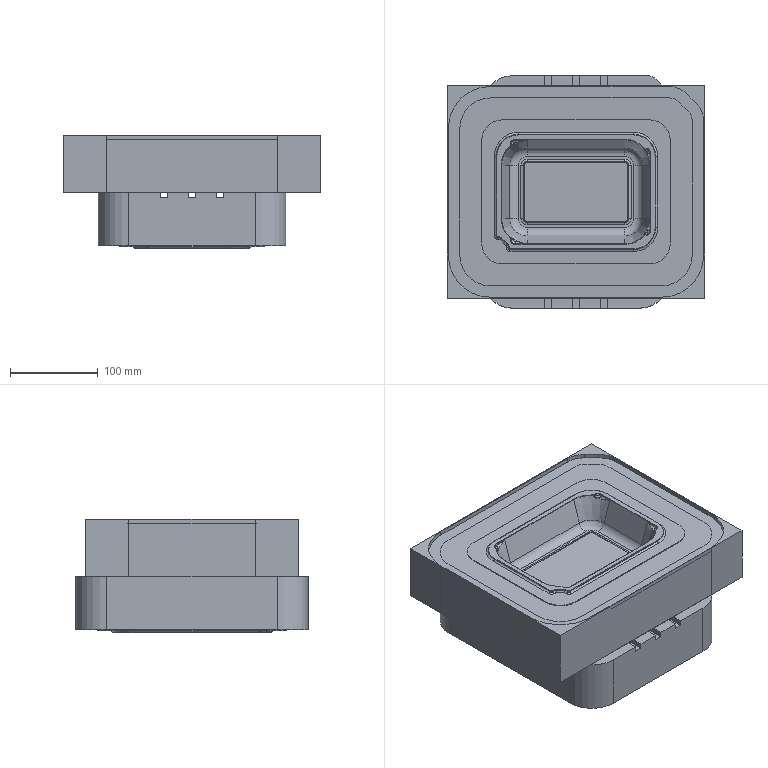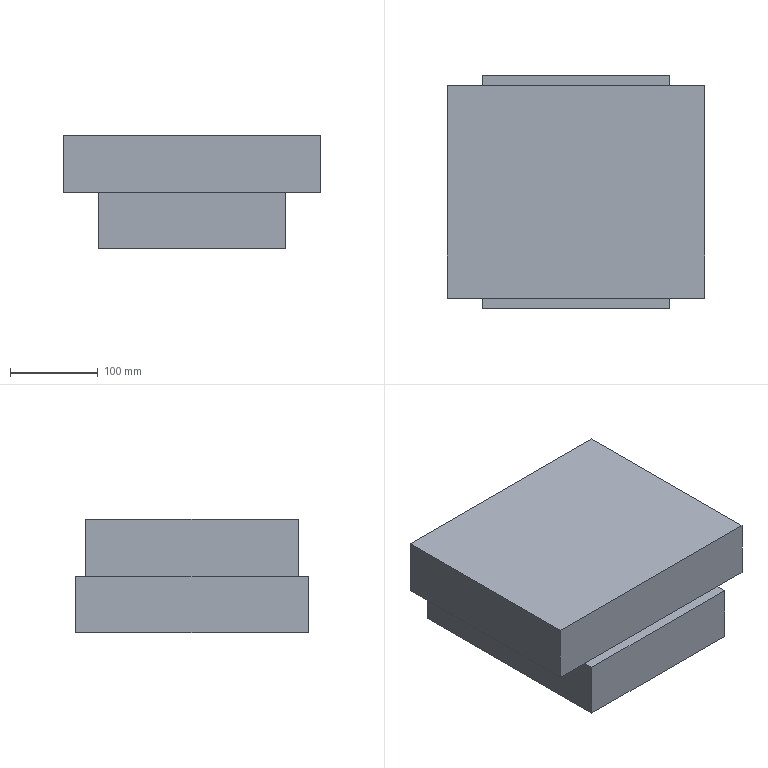CAM job | NX | 3-axis milling, drilling | part box 293.342 x 265.342 x 129.5 mm | stock box 293.342 x 265.342 x 129.5 mm
Tools:
number,name,description,diameter,corner_radius,flute_length,length,flutes
0,V2.0,Milling Tool-5 Parameters,2.0,1.0,30.0,30.0,4
0,V8.0,Drilling Tool,8.0,0.0,35.0,50.0,2
0,D12,No Description,12.0,0.0,50.0,70.0,2
0,D8,No Description,8.0,0.0,0.0,40.0,2
0,D16R0.8,No Description,16.0,0.8,50.0,90.0,2
0,R2,No Description,4.0,2.0,0.0,20.0,2
Operations:
program,operation,operation_type,tool,method,geometry_group,spindle_rpm,surface_speed,feed_per_tooth,feed_cut,feed_plunge,cut_length_mm,path_length_mm,cut_time_min,machine_time_min
B-1,B-,CavityMilling,D16R0.8,METHOD,22B,7000.0,1099.0,0.3214,4500.0,100.0,186040.168,191503.331,41.342,41.889
B-2,B2,CavityMilling,D8,METHOD,22B,7000.0,1099.0,0.3214,4500.0,100.0,13388.578,15465.942,2.975,3.183
B-3,B4,Engraving,R2,METHOD,22B,9000.0,14.0,0.0111,200.0,30.0,1128.732,10048.155,6.863,7.755
B-3,B5,SurfaceContour,R2,METHOD,22B,8000.0,251.0,0.2812,4500.0,100.0,165814.035,166146.976,36.848,36.881
B-4,DRILLING,Operation,V2.0,METHOD,22B,2000.0,75.0,0.0375,150.0,0.0,175.0,1875.194,1.167,1.337
B-5,B6,FaceMilling,D12,METHOD,22B,7000.0,1099.0,0.2857,4000.0,100.0,5079.431,5386.107,1.27,1.3
B-5,B7,PlanarMilling,D12,METHOD,22B,7000.0,571.0,0.2857,4000.0,100.0,71313.328,71681.416,17.828,17.865
C-1,CAVITY_MILL_1,CavityMilling,D8,METHOD,23C,7000.0,1099.0,0.3214,4500.0,100.0,80118.775,91046.234,17.804,18.897
C-2,DRILLING_1,Operation,V2.0,METHOD,23C,2000.0,75.0,0.0375,150.0,0.0,175.0,1817.991,1.167,1.331
C-3,DRILLING_2,Operation,V8.0,METHOD,23C,2000.0,75.0,0.0375,150.0,0.0,608.0,2142.345,4.053,4.207
C-3,DRILLING_2_COPY,Operation,V8.0,METHOD,23C,2000.0,75.0,0.0375,150.0,0.0,171.0,1169.566,1.14,1.24